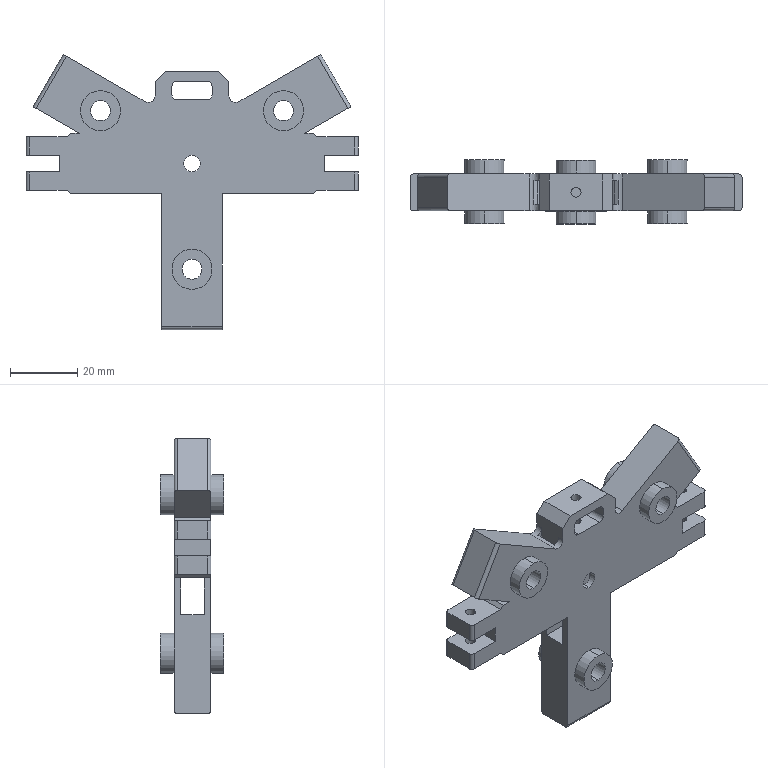Part | SolidWorks | features ICE 7, Revolution 6, Fillet 5, HoleWzd 5, MirrorPattern 5, Chamfer 1, Extrusion 1 | 1 solid | 114 faces | box 99 x 19 x 82.044 mm | volume 35178 mm3 | plane 58 | cylinder 56 | commonest cylinder face diameters 3 x16 2 x14 12 x12 6 x6 5 x4 4 x2